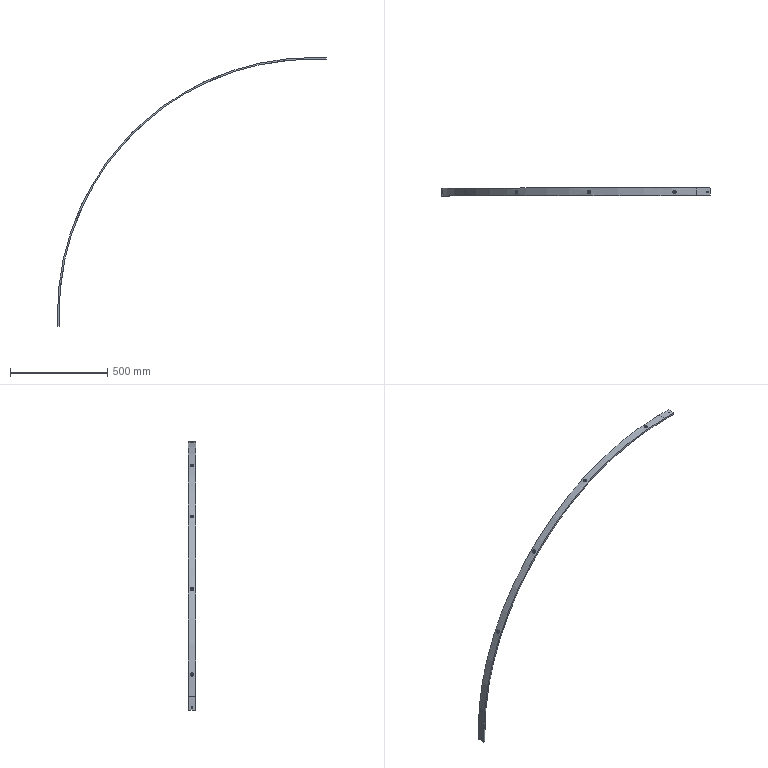Part | STEP file | for outer bend roller1 | 1 solid | 26 faces | box 1382 x 40 x 1382 mm | volume 697130 mm3 | plane 12 | spline 6 | cylinder 5 | cone 3 | commonest cylinder face diameters 9 x3 2608 x1 2624 x1